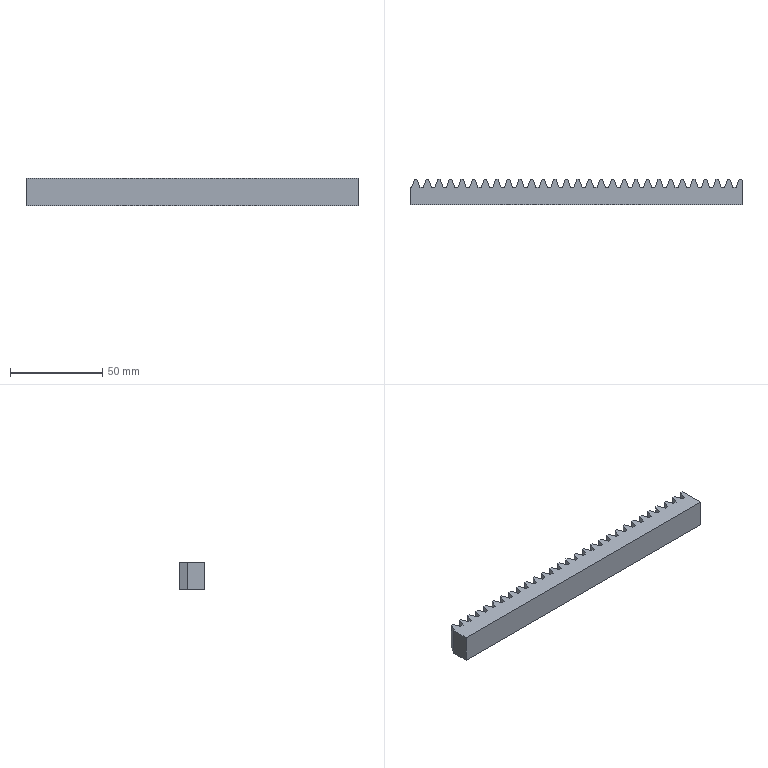Part | SolidWorks | features Cut 2, Extrusion 1, LPattern 1 | 1 solid | 121 faces | box 180 x 14 x 15 mm | volume 31331 mm3 | plane 121